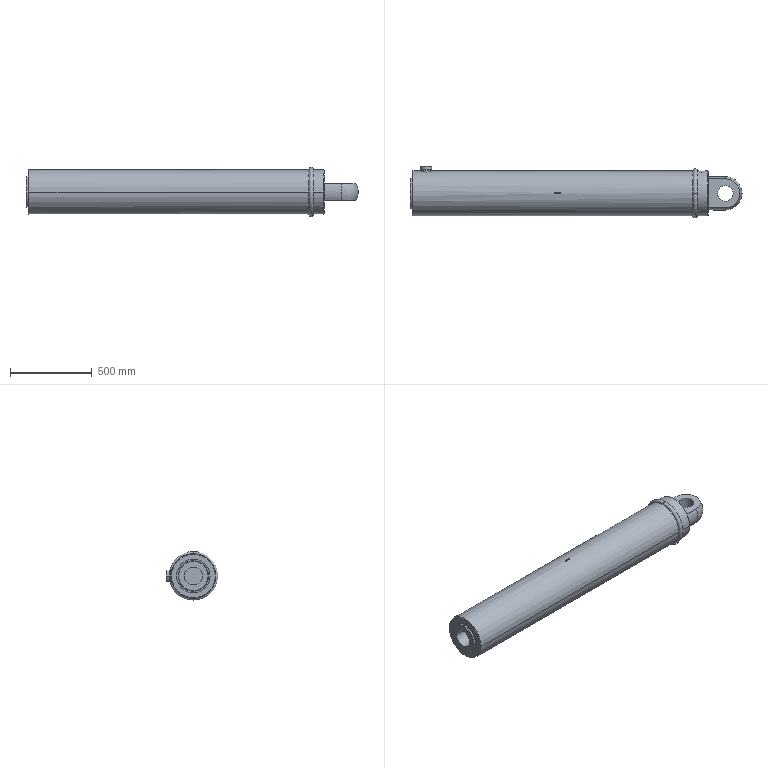Part | SolidWorks | features BaseBody 1 | 1 solid | 637 faces | box 2027 x 316.65 x 300.3 mm | volume 94983659 mm3 | plane 454 | spline 87 | cylinder 77 | cone 15 | sphere 2 | torus 2 | commonest cylinder face diameters 273.2 x48 273 x11 39.835 x4 67.2 x2 84 x2 95 x2